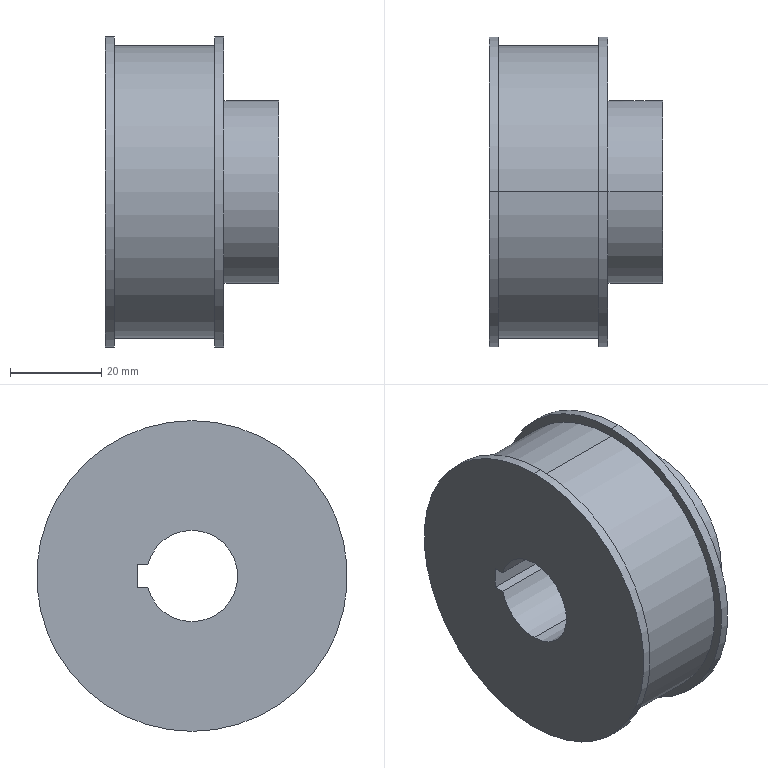Part | STEP file | PN_0001 (wheel) | 1 solid | 21 faces | box 38 x 68 x 68 mm | volume 87974 mm3 | cylinder 13 | plane 8 | commonest cylinder face diameters 68 x4 20 x3 3.3 x2 40 x2 64 x2